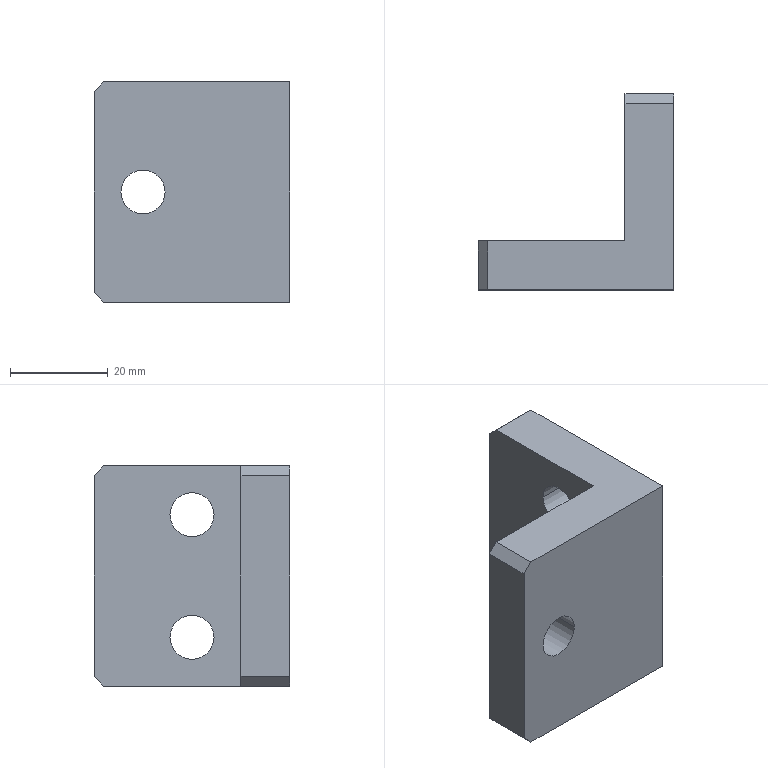Part | STEP file | 09-25 profile fixing bracket | 1 solid | 18 faces | box 40 x 40 x 45 mm | volume 29511 mm3 | plane 12 | cylinder 6 | commonest cylinder face diameters 9 x6
STEP:
#1=CARTESIAN_POINT('',(22.916,7.416,12.5));
#2=VERTEX_POINT('',#1);
#3=CARTESIAN_POINT('',(22.916,-1.584,12.5));
#4=VERTEX_POINT('',#3);
#5=CARTESIAN_POINT('',(22.916,2.916,12.5));
#6=DIRECTION('',(-1.,0.,0.));
#7=DIRECTION('',(0.,-1.,0.));
#8=AXIS2_PLACEMENT_3D('',#5,#6,#7);
#9=CIRCLE('',#8,4.5);
#10=EDGE_CURVE('',#2,#4,#9,.T.);
#11=ORIENTED_EDGE('',*,*,#10,.F.);
#12=CARTESIAN_POINT('',(12.916,7.416,12.5));
#13=VERTEX_POINT('',#12);
#14=CARTESIAN_POINT('',(77.916,7.416,12.5));
#15=DIRECTION('',(-1.,0.,0.));
#16=VECTOR('',#15,1000.);
#17=LINE('',#14,#16);
#18=EDGE_CURVE('',#2,#13,#17,.T.);
#19=ORIENTED_EDGE('',*,*,#18,.T.);
#20=CARTESIAN_POINT('',(12.916,-1.584,12.5));
#21=VERTEX_POINT('',#20);
#22=CARTESIAN_POINT('',(12.916,2.916,12.5));
#23=DIRECTION('',(-1.,0.,0.));
#24=DIRECTION('',(0.,1.,0.));
#25=AXIS2_PLACEMENT_3D('',#22,#23,#24);
#26=CIRCLE('',#25,4.5);
#27=EDGE_CURVE('',#13,#21,#26,.T.);
#28=ORIENTED_EDGE('',*,*,#27,.T.);
#29=CARTESIAN_POINT('',(77.916,-1.584,12.5));
#30=DIRECTION('',(-1.,0.,0.));
#31=VECTOR('',#30,1000.);
#32=LINE('',#29,#31);
#33=EDGE_CURVE('',#4,#21,#32,.T.);
#34=ORIENTED_EDGE('',*,*,#33,.F.);
#35=EDGE_LOOP('',(#11,#19,#28,#34));
#36=FACE_OUTER_BOUND('',#35,.T.);
#37=CARTESIAN_POINT('',(77.916,2.916,12.5));
#38=DIRECTION('',(-1.,0.,0.));
#39=DIRECTION('',(0.,-1.,0.));
#40=AXIS2_PLACEMENT_3D('',#37,#38,#39);
#41=CYLINDRICAL_SURFACE('',#40,4.5);
#42=ADVANCED_FACE('',(#36),#41,.F.);
#43=CARTESIAN_POINT('',(22.916,7.416,-12.5));
#44=VERTEX_POINT('',#43);
#45=CARTESIAN_POINT('',(22.916,-1.584,-12.5));
#46=VERTEX_POINT('',#45);
#47=CARTESIAN_POINT('',(22.916,2.916,-12.5));
#48=DIRECTION('',(-1.,0.,0.));
#49=DIRECTION('',(0.,-1.,0.));
#50=AXIS2_PLACEMENT_3D('',#47,#48,#49);
#51=CIRCLE('',#50,4.5);
#52=EDGE_CURVE('',#44,#46,#51,.T.);
#53=ORIENTED_EDGE('',*,*,#52,.F.);
#54=CARTESIAN_POINT('',(12.916,7.416,-12.5));
#55=VERTEX_POINT('',#54);
#56=CARTESIAN_POINT('',(77.916,7.416,-12.5));
#57=DIRECTION('',(-1.,0.,0.));
#58=VECTOR('',#57,1000.);
#59=LINE('',#56,#58);
#60=EDGE_CURVE('',#44,#55,#59,.T.);
#61=ORIENTED_EDGE('',*,*,#60,.T.);
#62=CARTESIAN_POINT('',(12.916,-1.584,-12.5));
#63=VERTEX_POINT('',#62);
#64=CARTESIAN_POINT('',(12.916,2.916,-12.5));
#65=DIRECTION('',(-1.,0.,0.));
#66=DIRECTION('',(0.,-1.,0.));
#67=AXIS2_PLACEMENT_3D('',#64,#65,#66);
#68=CIRCLE('',#67,4.5);
#69=EDGE_CURVE('',#55,#63,#68,.T.);
#70=ORIENTED_EDGE('',*,*,#69,.T.);
#71=CARTESIAN_POINT('',(77.916,-1.584,-12.5));
#72=DIRECTION('',(-1.,0.,0.));
#73=VECTOR('',#72,1000.);
#74=LINE('',#71,#73);
#75=EDGE_CURVE('',#46,#63,#74,.T.);
#76=ORIENTED_EDGE('',*,*,#75,.F.);
#77=EDGE_LOOP('',(#53,#61,#70,#76));
#78=FACE_OUTER_BOUND('',#77,.T.);
#79=CARTESIAN_POINT('',(77.916,2.916,-12.5));
#80=DIRECTION('',(-1.,0.,0.));
#81=DIRECTION('',(0.,-1.,0.));
#82=AXIS2_PLACEMENT_3D('',#79,#80,#81);
#83=CYLINDRICAL_SURFACE('',#82,4.5);
#84=ADVANCED_FACE('',(#78),#83,.F.);
#85=CARTESIAN_POINT('',(-2.584,-17.084,0.));
#86=VERTEX_POINT('',#85);
#87=CARTESIAN_POINT('',(-11.584,-17.084,0.));
#88=VERTEX_POINT('',#87);
#89=CARTESIAN_POINT('',(-7.084,-17.084,0.));
#90=DIRECTION('',(0.,1.,0.));
#91=DIRECTION('',(0.,0.,1.));
#92=AXIS2_PLACEMENT_3D('',#89,#90,#91);
#93=CIRCLE('',#92,4.5);
#94=EDGE_CURVE('',#86,#88,#93,.T.);
#95=ORIENTED_EDGE('',*,*,#94,.F.);
#96=CARTESIAN_POINT('',(-2.584,-7.084,0.));
#97=VERTEX_POINT('',#96);
#98=CARTESIAN_POINT('',(-2.584,-72.084,0.));
#99=DIRECTION('',(0.,1.,0.));
#100=VECTOR('',#99,1000.);
#101=LINE('',#98,#100);
#102=EDGE_CURVE('',#86,#97,#101,.T.);
#103=ORIENTED_EDGE('',*,*,#102,.T.);
#104=CARTESIAN_POINT('',(-11.584,-7.084,0.));
#105=VERTEX_POINT('',#104);
#106=CARTESIAN_POINT('',(-7.084,-7.084,0.));
#107=DIRECTION('',(0.,1.,0.));
#108=DIRECTION('',(-1.,0.,0.));
#109=AXIS2_PLACEMENT_3D('',#106,#107,#108);
#110=CIRCLE('',#109,4.5);
#111=EDGE_CURVE('',#97,#105,#110,.T.);
#112=ORIENTED_EDGE('',*,*,#111,.T.);
#113=CARTESIAN_POINT('',(-11.584,-72.084,0.));
#114=DIRECTION('',(0.,1.,0.));
#115=VECTOR('',#114,1000.);
#116=LINE('',#113,#115);
#117=EDGE_CURVE('',#88,#105,#116,.T.);
#118=ORIENTED_EDGE('',*,*,#117,.F.);
#119=EDGE_LOOP('',(#95,#103,#112,#118));
#120=FACE_OUTER_BOUND('',#119,.T.);
#121=CARTESIAN_POINT('',(-7.084,-72.084,0.));
#122=DIRECTION('',(0.,1.,0.));
#123=DIRECTION('',(-1.,0.,0.));
#124=AXIS2_PLACEMENT_3D('',#121,#122,#123);
#125=CYLINDRICAL_SURFACE('',#124,4.5);
#126=ADVANCED_FACE('',(#120),#125,.F.);
#127=CARTESIAN_POINT('',(22.916,2.916,12.5));
#128=DIRECTION('',(-1.,0.,0.));
#129=DIRECTION('',(0.,-1.,0.));
#130=AXIS2_PLACEMENT_3D('',#127,#128,#129);
#131=CIRCLE('',#130,4.5);
#132=EDGE_CURVE('',#4,#2,#131,.T.);
#133=ORIENTED_EDGE('',*,*,#132,.T.);
#134=ORIENTED_EDGE('',*,*,#10,.T.);
#135=EDGE_LOOP('',(#133,#134));
#136=FACE_BOUND('',#135,.T.);
#137=CARTESIAN_POINT('',(22.916,2.916,-12.5));
#138=DIRECTION('',(-1.,0.,0.));
#139=DIRECTION('',(0.,-1.,0.));
#140=AXIS2_PLACEMENT_3D('',#137,#138,#139);
#141=CIRCLE('',#140,4.5);
#142=EDGE_CURVE('',#46,#44,#141,.T.);
#143=ORIENTED_EDGE('',*,*,#142,.T.);
#144=ORIENTED_EDGE('',*,*,#52,.T.);
#145=EDGE_LOOP('',(#143,#144));
#146=FACE_BOUND('',#145,.T.);
#147=CARTESIAN_POINT('',(22.916,22.916,20.5));
#148=VERTEX_POINT('',#147);
#149=CARTESIAN_POINT('',(22.916,22.916,-20.5));
#150=VERTEX_POINT('',#149);
#151=CARTESIAN_POINT('',(22.916,22.916,22.5));
#152=DIRECTION('',(0.,0.,-1.));
#153=VECTOR('',#152,1000.);
#154=LINE('',#151,#153);
#155=EDGE_CURVE('',#148,#150,#154,.T.);
#156=ORIENTED_EDGE('',*,*,#155,.F.);
#157=CARTESIAN_POINT('',(22.916,20.916,22.5));
#158=VERTEX_POINT('',#157);
#159=CARTESIAN_POINT('',(22.916,20.916,22.5));
#160=DIRECTION('',(0.,-0.7071,0.7071));
#161=VECTOR('',#160,1000.);
#162=LINE('',#159,#161);
#163=EDGE_CURVE('',#148,#158,#162,.T.);
#164=ORIENTED_EDGE('',*,*,#163,.T.);
#165=CARTESIAN_POINT('',(22.916,-17.084,22.5));
#166=VERTEX_POINT('',#165);
#167=CARTESIAN_POINT('',(22.916,22.916,22.5));
#168=DIRECTION('',(0.,1.,0.));
#169=VECTOR('',#168,1000.);
#170=LINE('',#167,#169);
#171=EDGE_CURVE('',#166,#158,#170,.T.);
#172=ORIENTED_EDGE('',*,*,#171,.F.);
#173=CARTESIAN_POINT('',(22.916,-17.084,-22.5));
#174=VERTEX_POINT('',#173);
#175=CARTESIAN_POINT('',(22.916,-17.084,22.5));
#176=DIRECTION('',(0.,0.,-1.));
#177=VECTOR('',#176,1000.);
#178=LINE('',#175,#177);
#179=EDGE_CURVE('',#166,#174,#178,.T.);
#180=ORIENTED_EDGE('',*,*,#179,.T.);
#181=CARTESIAN_POINT('',(22.916,20.916,-22.5));
#182=VERTEX_POINT('',#181);
#183=CARTESIAN_POINT('',(22.916,22.916,-22.5));
#184=DIRECTION('',(0.,1.,0.));
#185=VECTOR('',#184,1000.);
#186=LINE('',#183,#185);
#187=EDGE_CURVE('',#174,#182,#186,.T.);
#188=ORIENTED_EDGE('',*,*,#187,.T.);
#189=CARTESIAN_POINT('',(22.916,22.916,-20.5));
#190=DIRECTION('',(0.,0.7071,0.7071));
#191=VECTOR('',#190,1000.);
#192=LINE('',#189,#191);
#193=EDGE_CURVE('',#182,#150,#192,.T.);
#194=ORIENTED_EDGE('',*,*,#193,.T.);
#195=EDGE_LOOP('',(#156,#164,#172,#180,#188,#194));
#196=FACE_OUTER_BOUND('',#195,.T.);
#197=CARTESIAN_POINT('',(22.916,22.916,22.5));
#198=DIRECTION('',(-1.,0.,0.));
#199=DIRECTION('',(0.,-1.,0.));
#200=AXIS2_PLACEMENT_3D('',#197,#198,#199);
#201=PLANE('',#200);
#202=ADVANCED_FACE('',(#136,#146,#196),#201,.F.);
#203=CARTESIAN_POINT('',(12.916,22.916,20.5));
#204=VERTEX_POINT('',#203);
#205=CARTESIAN_POINT('',(12.916,22.916,-20.5));
#206=VERTEX_POINT('',#205);
#207=CARTESIAN_POINT('',(12.916,22.916,22.5));
#208=DIRECTION('',(0.,0.,-1.));
#209=VECTOR('',#208,1000.);
#210=LINE('',#207,#209);
#211=EDGE_CURVE('',#204,#206,#210,.T.);
#212=ORIENTED_EDGE('',*,*,#211,.F.);
#213=CARTESIAN_POINT('',(22.916,22.916,20.5));
#214=DIRECTION('',(1.,0.,0.));
#215=VECTOR('',#214,1000.);
#216=LINE('',#213,#215);
#217=EDGE_CURVE('',#204,#148,#216,.T.);
#218=ORIENTED_EDGE('',*,*,#217,.T.);
#219=ORIENTED_EDGE('',*,*,#155,.T.);
#220=CARTESIAN_POINT('',(12.916,22.916,-20.5));
#221=DIRECTION('',(-1.,0.,0.));
#222=VECTOR('',#221,1000.);
#223=LINE('',#220,#222);
#224=EDGE_CURVE('',#150,#206,#223,.T.);
#225=ORIENTED_EDGE('',*,*,#224,.T.);
#226=EDGE_LOOP('',(#212,#218,#219,#225));
#227=FACE_OUTER_BOUND('',#226,.T.);
#228=CARTESIAN_POINT('',(12.916,22.916,22.5));
#229=DIRECTION('',(0.,-1.,0.));
#230=DIRECTION('',(0.,0.,-1.));
#231=AXIS2_PLACEMENT_3D('',#228,#229,#230);
#232=PLANE('',#231);
#233=ADVANCED_FACE('',(#227),#232,.F.);
#234=CARTESIAN_POINT('',(12.916,2.916,12.5));
#235=DIRECTION('',(-1.,0.,0.));
#236=DIRECTION('',(0.,1.,0.));
#237=AXIS2_PLACEMENT_3D('',#234,#235,#236);
#238=CIRCLE('',#237,4.5);
#239=EDGE_CURVE('',#21,#13,#238,.T.);
#240=ORIENTED_EDGE('',*,*,#239,.F.);
#241=ORIENTED_EDGE('',*,*,#27,.F.);
#242=EDGE_LOOP('',(#240,#241));
#243=FACE_BOUND('',#242,.T.);
#244=CARTESIAN_POINT('',(12.916,2.916,-12.5));
#245=DIRECTION('',(-1.,0.,0.));
#246=DIRECTION('',(0.,-1.,0.));
#247=AXIS2_PLACEMENT_3D('',#244,#245,#246);
#248=CIRCLE('',#247,4.5);
#249=EDGE_CURVE('',#63,#55,#248,.T.);
#250=ORIENTED_EDGE('',*,*,#249,.F.);
#251=ORIENTED_EDGE('',*,*,#69,.F.);
#252=EDGE_LOOP('',(#250,#251));
#253=FACE_BOUND('',#252,.T.);
#254=CARTESIAN_POINT('',(12.916,20.916,22.5));
#255=VERTEX_POINT('',#254);
#256=CARTESIAN_POINT('',(12.916,-7.084,22.5));
#257=VERTEX_POINT('',#256);
#258=CARTESIAN_POINT('',(12.916,22.916,22.5));
#259=DIRECTION('',(0.,-1.,0.));
#260=VECTOR('',#259,1000.);
#261=LINE('',#258,#260);
#262=EDGE_CURVE('',#255,#257,#261,.T.);
#263=ORIENTED_EDGE('',*,*,#262,.F.);
#264=CARTESIAN_POINT('',(12.916,20.916,22.5));
#265=DIRECTION('',(0.,0.7071,-0.7071));
#266=VECTOR('',#265,1000.);
#267=LINE('',#264,#266);
#268=EDGE_CURVE('',#255,#204,#267,.T.);
#269=ORIENTED_EDGE('',*,*,#268,.T.);
#270=ORIENTED_EDGE('',*,*,#211,.T.);
#271=CARTESIAN_POINT('',(12.916,20.916,-22.5));
#272=VERTEX_POINT('',#271);
#273=CARTESIAN_POINT('',(12.916,22.916,-20.5));
#274=DIRECTION('',(0.,-0.7071,-0.7071));
#275=VECTOR('',#274,1000.);
#276=LINE('',#273,#275);
#277=EDGE_CURVE('',#206,#272,#276,.T.);
#278=ORIENTED_EDGE('',*,*,#277,.T.);
#279=CARTESIAN_POINT('',(12.916,-7.084,-22.5));
#280=VERTEX_POINT('',#279);
#281=CARTESIAN_POINT('',(12.916,22.916,-22.5));
#282=DIRECTION('',(0.,-1.,0.));
#283=VECTOR('',#282,1000.);
#284=LINE('',#281,#283);
#285=EDGE_CURVE('',#272,#280,#284,.T.);
#286=ORIENTED_EDGE('',*,*,#285,.T.);
#287=CARTESIAN_POINT('',(12.916,-7.084,22.5));
#288=DIRECTION('',(0.,0.,-1.));
#289=VECTOR('',#288,1000.);
#290=LINE('',#287,#289);
#291=EDGE_CURVE('',#257,#280,#290,.T.);
#292=ORIENTED_EDGE('',*,*,#291,.F.);
#293=EDGE_LOOP('',(#263,#269,#270,#278,#286,#292));
#294=FACE_OUTER_BOUND('',#293,.T.);
#295=CARTESIAN_POINT('',(12.916,22.916,22.5));
#296=DIRECTION('',(1.,0.,0.));
#297=DIRECTION('',(0.,1.,0.));
#298=AXIS2_PLACEMENT_3D('',#295,#296,#297);
#299=PLANE('',#298);
#300=ADVANCED_FACE('',(#243,#253,#294),#299,.F.);
#301=CARTESIAN_POINT('',(-7.084,-7.084,0.));
#302=DIRECTION('',(0.,1.,0.));
#303=DIRECTION('',(-1.,0.,0.));
#304=AXIS2_PLACEMENT_3D('',#301,#302,#303);
#305=CIRCLE('',#304,4.5);
#306=EDGE_CURVE('',#105,#97,#305,.T.);
#307=ORIENTED_EDGE('',*,*,#306,.F.);
#308=ORIENTED_EDGE('',*,*,#111,.F.);
#309=EDGE_LOOP('',(#307,#308));
#310=FACE_BOUND('',#309,.T.);
#311=CARTESIAN_POINT('',(-17.084,-7.084,20.5));
#312=VERTEX_POINT('',#311);
#313=CARTESIAN_POINT('',(-17.084,-7.084,-20.5));
#314=VERTEX_POINT('',#313);
#315=CARTESIAN_POINT('',(-17.084,-7.084,22.5));
#316=DIRECTION('',(0.,0.,-1.));
#317=VECTOR('',#316,1000.);
#318=LINE('',#315,#317);
#319=EDGE_CURVE('',#312,#314,#318,.T.);
#320=ORIENTED_EDGE('',*,*,#319,.F.);
#321=CARTESIAN_POINT('',(-15.084,-7.084,22.5));
#322=VERTEX_POINT('',#321);
#323=CARTESIAN_POINT('',(-15.084,-7.084,22.5));
#324=DIRECTION('',(0.7071,0.,0.7071));
#325=VECTOR('',#324,1000.);
#326=LINE('',#323,#325);
#327=EDGE_CURVE('',#312,#322,#326,.T.);
#328=ORIENTED_EDGE('',*,*,#327,.T.);
#329=CARTESIAN_POINT('',(-17.084,-7.084,22.5));
#330=DIRECTION('',(-1.,0.,0.));
#331=VECTOR('',#330,1000.);
#332=LINE('',#329,#331);
#333=EDGE_CURVE('',#257,#322,#332,.T.);
#334=ORIENTED_EDGE('',*,*,#333,.F.);
#335=ORIENTED_EDGE('',*,*,#291,.T.);
#336=CARTESIAN_POINT('',(-15.084,-7.084,-22.5));
#337=VERTEX_POINT('',#336);
#338=CARTESIAN_POINT('',(-17.084,-7.084,-22.5));
#339=DIRECTION('',(-1.,0.,0.));
#340=VECTOR('',#339,1000.);
#341=LINE('',#338,#340);
#342=EDGE_CURVE('',#280,#337,#341,.T.);
#343=ORIENTED_EDGE('',*,*,#342,.T.);
#344=CARTESIAN_POINT('',(-17.084,-7.084,-20.5));
#345=DIRECTION('',(-0.7071,0.,0.7071));
#346=VECTOR('',#345,1000.);
#347=LINE('',#344,#346);
#348=EDGE_CURVE('',#337,#314,#347,.T.);
#349=ORIENTED_EDGE('',*,*,#348,.T.);
#350=EDGE_LOOP('',(#320,#328,#334,#335,#343,#349));
#351=FACE_OUTER_BOUND('',#350,.T.);
#352=CARTESIAN_POINT('',(-17.084,-7.084,22.5));
#353=DIRECTION('',(0.,-1.,0.));
#354=DIRECTION('',(0.,0.,-1.));
#355=AXIS2_PLACEMENT_3D('',#352,#353,#354);
#356=PLANE('',#355);
#357=ADVANCED_FACE('',(#310,#351),#356,.F.);
#358=CARTESIAN_POINT('',(-17.084,-17.084,20.5));
#359=VERTEX_POINT('',#358);
#360=CARTESIAN_POINT('',(-17.084,-17.084,-20.5));
#361=VERTEX_POINT('',#360);
#362=CARTESIAN_POINT('',(-17.084,-17.084,22.5));
#363=DIRECTION('',(0.,0.,-1.));
#364=VECTOR('',#363,1000.);
#365=LINE('',#362,#364);
#366=EDGE_CURVE('',#359,#361,#365,.T.);
#367=ORIENTED_EDGE('',*,*,#366,.F.);
#368=CARTESIAN_POINT('',(-17.084,-7.084,20.5));
#369=DIRECTION('',(0.,1.,0.));
#370=VECTOR('',#369,1000.);
#371=LINE('',#368,#370);
#372=EDGE_CURVE('',#359,#312,#371,.T.);
#373=ORIENTED_EDGE('',*,*,#372,.T.);
#374=ORIENTED_EDGE('',*,*,#319,.T.);
#375=CARTESIAN_POINT('',(-17.084,-7.084,-20.5));
#376=DIRECTION('',(0.,-1.,0.));
#377=VECTOR('',#376,1000.);
#378=LINE('',#375,#377);
#379=EDGE_CURVE('',#314,#361,#378,.T.);
#380=ORIENTED_EDGE('',*,*,#379,.T.);
#381=EDGE_LOOP('',(#367,#373,#374,#380));
#382=FACE_OUTER_BOUND('',#381,.T.);
#383=CARTESIAN_POINT('',(-17.084,-7.084,22.5));
#384=DIRECTION('',(1.,0.,0.));
#385=DIRECTION('',(0.,1.,0.));
#386=AXIS2_PLACEMENT_3D('',#383,#384,#385);
#387=PLANE('',#386);
#388=ADVANCED_FACE('',(#382),#387,.F.);
#389=CARTESIAN_POINT('',(-7.084,-17.084,0.));
#390=DIRECTION('',(0.,1.,0.));
#391=DIRECTION('',(0.,0.,1.));
#392=AXIS2_PLACEMENT_3D('',#389,#390,#391);
#393=CIRCLE('',#392,4.5);
#394=EDGE_CURVE('',#88,#86,#393,.T.);
#395=ORIENTED_EDGE('',*,*,#394,.T.);
#396=ORIENTED_EDGE('',*,*,#94,.T.);
#397=EDGE_LOOP('',(#395,#396));
#398=FACE_BOUND('',#397,.T.);
#399=CARTESIAN_POINT('',(-15.084,-17.084,22.5));
#400=VERTEX_POINT('',#399);
#401=CARTESIAN_POINT('',(-17.084,-17.084,22.5));
#402=DIRECTION('',(1.,0.,0.));
#403=VECTOR('',#402,1000.);
#404=LINE('',#401,#403);
#405=EDGE_CURVE('',#400,#166,#404,.T.);
#406=ORIENTED_EDGE('',*,*,#405,.F.);
#407=CARTESIAN_POINT('',(-15.084,-17.084,22.5));
#408=DIRECTION('',(-0.7071,0.,-0.7071));
#409=VECTOR('',#408,1000.);
#410=LINE('',#407,#409);
#411=EDGE_CURVE('',#400,#359,#410,.T.);
#412=ORIENTED_EDGE('',*,*,#411,.T.);
#413=ORIENTED_EDGE('',*,*,#366,.T.);
#414=CARTESIAN_POINT('',(-15.084,-17.084,-22.5));
#415=VERTEX_POINT('',#414);
#416=CARTESIAN_POINT('',(-17.084,-17.084,-20.5));
#417=DIRECTION('',(0.7071,0.,-0.7071));
#418=VECTOR('',#417,1000.);
#419=LINE('',#416,#418);
#420=EDGE_CURVE('',#361,#415,#419,.T.);
#421=ORIENTED_EDGE('',*,*,#420,.T.);
#422=CARTESIAN_POINT('',(-17.084,-17.084,-22.5));
#423=DIRECTION('',(1.,0.,0.));
#424=VECTOR('',#423,1000.);
#425=LINE('',#422,#424);
#426=EDGE_CURVE('',#415,#174,#425,.T.);
#427=ORIENTED_EDGE('',*,*,#426,.T.);
#428=ORIENTED_EDGE('',*,*,#179,.F.);
#429=EDGE_LOOP('',(#406,#412,#413,#421,#427,#428));
#430=FACE_OUTER_BOUND('',#429,.T.);
#431=CARTESIAN_POINT('',(-17.084,-17.084,22.5));
#432=DIRECTION('',(0.,1.,0.));
#433=DIRECTION('',(0.,0.,1.));
#434=AXIS2_PLACEMENT_3D('',#431,#432,#433);
#435=PLANE('',#434);
#436=ADVANCED_FACE('',(#398,#430),#435,.F.);
#437=ORIENTED_EDGE('',*,*,#171,.T.);
#438=CARTESIAN_POINT('',(12.916,20.916,22.5));
#439=DIRECTION('',(-1.,0.,0.));
#440=VECTOR('',#439,1000.);
#441=LINE('',#438,#440);
#442=EDGE_CURVE('',#158,#255,#441,.T.);
#443=ORIENTED_EDGE('',*,*,#442,.T.);
#444=ORIENTED_EDGE('',*,*,#262,.T.);
#445=ORIENTED_EDGE('',*,*,#333,.T.);
#446=CARTESIAN_POINT('',(-15.084,-17.084,22.5));
#447=DIRECTION('',(0.,-1.,0.));
#448=VECTOR('',#447,1000.);
#449=LINE('',#446,#448);
#450=EDGE_CURVE('',#322,#400,#449,.T.);
#451=ORIENTED_EDGE('',*,*,#450,.T.);
#452=ORIENTED_EDGE('',*,*,#405,.T.);
#453=EDGE_LOOP('',(#437,#443,#444,#445,#451,#452));
#454=FACE_OUTER_BOUND('',#453,.T.);
#455=CARTESIAN_POINT('',(22.916,-17.084,22.5));
#456=DIRECTION('',(0.,0.,1.));
#457=DIRECTION('',(1.,0.,0.));
#458=AXIS2_PLACEMENT_3D('',#455,#456,#457);
#459=PLANE('',#458);
#460=ADVANCED_FACE('',(#454),#459,.T.);
#461=ORIENTED_EDGE('',*,*,#285,.F.);
#462=CARTESIAN_POINT('',(22.916,20.916,-22.5));
#463=DIRECTION('',(1.,0.,0.));
#464=VECTOR('',#463,1000.);
#465=LINE('',#462,#464);
#466=EDGE_CURVE('',#272,#182,#465,.T.);
#467=ORIENTED_EDGE('',*,*,#466,.T.);
#468=ORIENTED_EDGE('',*,*,#187,.F.);
#469=ORIENTED_EDGE('',*,*,#426,.F.);
#470=CARTESIAN_POINT('',(-15.084,-17.084,-22.5));
#471=DIRECTION('',(0.,1.,0.));
#472=VECTOR('',#471,1000.);
#473=LINE('',#470,#472);
#474=EDGE_CURVE('',#415,#337,#473,.T.);
#475=ORIENTED_EDGE('',*,*,#474,.T.);
#476=ORIENTED_EDGE('',*,*,#342,.F.);
#477=EDGE_LOOP('',(#461,#467,#468,#469,#475,#476));
#478=FACE_OUTER_BOUND('',#477,.T.);
#479=CARTESIAN_POINT('',(22.916,-17.084,-22.5));
#480=DIRECTION('',(0.,0.,1.));
#481=DIRECTION('',(1.,0.,0.));
#482=AXIS2_PLACEMENT_3D('',#479,#480,#481);
#483=PLANE('',#482);
#484=ADVANCED_FACE('',(#478),#483,.F.);
#485=ORIENTED_EDGE('',*,*,#102,.F.);
#486=ORIENTED_EDGE('',*,*,#394,.F.);
#487=ORIENTED_EDGE('',*,*,#117,.T.);
#488=ORIENTED_EDGE('',*,*,#306,.T.);
#489=EDGE_LOOP('',(#485,#486,#487,#488));
#490=FACE_OUTER_BOUND('',#489,.T.);
#491=CARTESIAN_POINT('',(-7.084,-72.084,0.));
#492=DIRECTION('',(0.,1.,0.));
#493=DIRECTION('',(-1.,0.,0.));
#494=AXIS2_PLACEMENT_3D('',#491,#492,#493);
#495=CYLINDRICAL_SURFACE('',#494,4.5);
#496=ADVANCED_FACE('',(#490),#495,.F.);
#497=ORIENTED_EDGE('',*,*,#60,.F.);
#498=ORIENTED_EDGE('',*,*,#142,.F.);
#499=ORIENTED_EDGE('',*,*,#75,.T.);
#500=ORIENTED_EDGE('',*,*,#249,.T.);
#501=EDGE_LOOP('',(#497,#498,#499,#500));
#502=FACE_OUTER_BOUND('',#501,.T.);
#503=CARTESIAN_POINT('',(77.916,2.916,-12.5));
#504=DIRECTION('',(-1.,0.,0.));
#505=DIRECTION('',(0.,-1.,0.));
#506=AXIS2_PLACEMENT_3D('',#503,#504,#505);
#507=CYLINDRICAL_SURFACE('',#506,4.5);
#508=ADVANCED_FACE('',(#502),#507,.F.);
#509=ORIENTED_EDGE('',*,*,#18,.F.);
#510=ORIENTED_EDGE('',*,*,#132,.F.);
#511=ORIENTED_EDGE('',*,*,#33,.T.);
#512=ORIENTED_EDGE('',*,*,#239,.T.);
#513=EDGE_LOOP('',(#509,#510,#511,#512));
#514=FACE_OUTER_BOUND('',#513,.T.);
#515=CARTESIAN_POINT('',(77.916,2.916,12.5));
#516=DIRECTION('',(-1.,0.,0.));
#517=DIRECTION('',(0.,-1.,0.));
#518=AXIS2_PLACEMENT_3D('',#515,#516,#517);
#519=CYLINDRICAL_SURFACE('',#518,4.5);
#520=ADVANCED_FACE('',(#514),#519,.F.);
#521=ORIENTED_EDGE('',*,*,#163,.F.);
#522=ORIENTED_EDGE('',*,*,#217,.F.);
#523=ORIENTED_EDGE('',*,*,#268,.F.);
#524=ORIENTED_EDGE('',*,*,#442,.F.);
#525=EDGE_LOOP('',(#521,#522,#523,#524));
#526=FACE_OUTER_BOUND('',#525,.T.);
#527=CARTESIAN_POINT('',(22.916,20.916,22.5));
#528=DIRECTION('',(0.,0.7071,0.7071));
#529=DIRECTION('',(0.,-0.7071,0.7071));
#530=AXIS2_PLACEMENT_3D('',#527,#528,#529);
#531=PLANE('',#530);
#532=ADVANCED_FACE('',(#526),#531,.T.);
#533=ORIENTED_EDGE('',*,*,#193,.F.);
#534=ORIENTED_EDGE('',*,*,#466,.F.);
#535=ORIENTED_EDGE('',*,*,#277,.F.);
#536=ORIENTED_EDGE('',*,*,#224,.F.);
#537=EDGE_LOOP('',(#533,#534,#535,#536));
#538=FACE_OUTER_BOUND('',#537,.T.);
#539=CARTESIAN_POINT('',(12.916,22.916,-20.5));
#540=DIRECTION('',(0.,-0.7071,0.7071));
#541=DIRECTION('',(0.,-0.7071,-0.7071));
#542=AXIS2_PLACEMENT_3D('',#539,#540,#541);
#543=PLANE('',#542);
#544=ADVANCED_FACE('',(#538),#543,.F.);
#545=ORIENTED_EDGE('',*,*,#327,.F.);
#546=ORIENTED_EDGE('',*,*,#372,.F.);
#547=ORIENTED_EDGE('',*,*,#411,.F.);
#548=ORIENTED_EDGE('',*,*,#450,.F.);
#549=EDGE_LOOP('',(#545,#546,#547,#548));
#550=FACE_OUTER_BOUND('',#549,.T.);
#551=CARTESIAN_POINT('',(-15.084,-17.084,22.5));
#552=DIRECTION('',(-0.7071,0.,0.7071));
#553=DIRECTION('',(0.7071,0.,0.7071));
#554=AXIS2_PLACEMENT_3D('',#551,#552,#553);
#555=PLANE('',#554);
#556=ADVANCED_FACE('',(#550),#555,.T.);
#557=ORIENTED_EDGE('',*,*,#348,.F.);
#558=ORIENTED_EDGE('',*,*,#474,.F.);
#559=ORIENTED_EDGE('',*,*,#420,.F.);
#560=ORIENTED_EDGE('',*,*,#379,.F.);
#561=EDGE_LOOP('',(#557,#558,#559,#560));
#562=FACE_OUTER_BOUND('',#561,.T.);
#563=CARTESIAN_POINT('',(-17.084,-7.084,-20.5));
#564=DIRECTION('',(0.7071,0.,0.7071));
#565=DIRECTION('',(0.7071,0.,-0.7071));
#566=AXIS2_PLACEMENT_3D('',#563,#564,#565);
#567=PLANE('',#566);
#568=ADVANCED_FACE('',(#562),#567,.F.);
#569=CLOSED_SHELL('',(#42,#84,#126,#202,#233,#300,#357,#388,#436,#460,#484,#496,#508,#520,#532,#544,#556,#568));
#570=MANIFOLD_SOLID_BREP('',#569);
#571=CARTESIAN_POINT('',(0.,0.,0.));
#572=DIRECTION('',(0.,0.,1.));
#573=DIRECTION('',(1.,0.,0.));
#574=AXIS2_PLACEMENT_3D('',#571,#572,#573);
#575=(LENGTH_UNIT()NAMED_UNIT(*)SI_UNIT(.MILLI.,.METRE.));
#576=UNCERTAINTY_MEASURE_WITH_UNIT(LENGTH_MEASURE(0.00001),#575,'','');
#577=(NAMED_UNIT(*)PLANE_ANGLE_UNIT()SI_UNIT($,.RADIAN.));
#578=(NAMED_UNIT(*)SI_UNIT($,.STERADIAN.)SOLID_ANGLE_UNIT());
#579=(GEOMETRIC_REPRESENTATION_CONTEXT(3)GLOBAL_UNCERTAINTY_ASSIGNED_CONTEXT((#576))GLOBAL_UNIT_ASSIGNED_CONTEXT((#575,#577,#578))REPRESENTATION_CONTEXT('',''));
#580=ADVANCED_BREP_SHAPE_REPRESENTATION('',(#570,#574),#579);